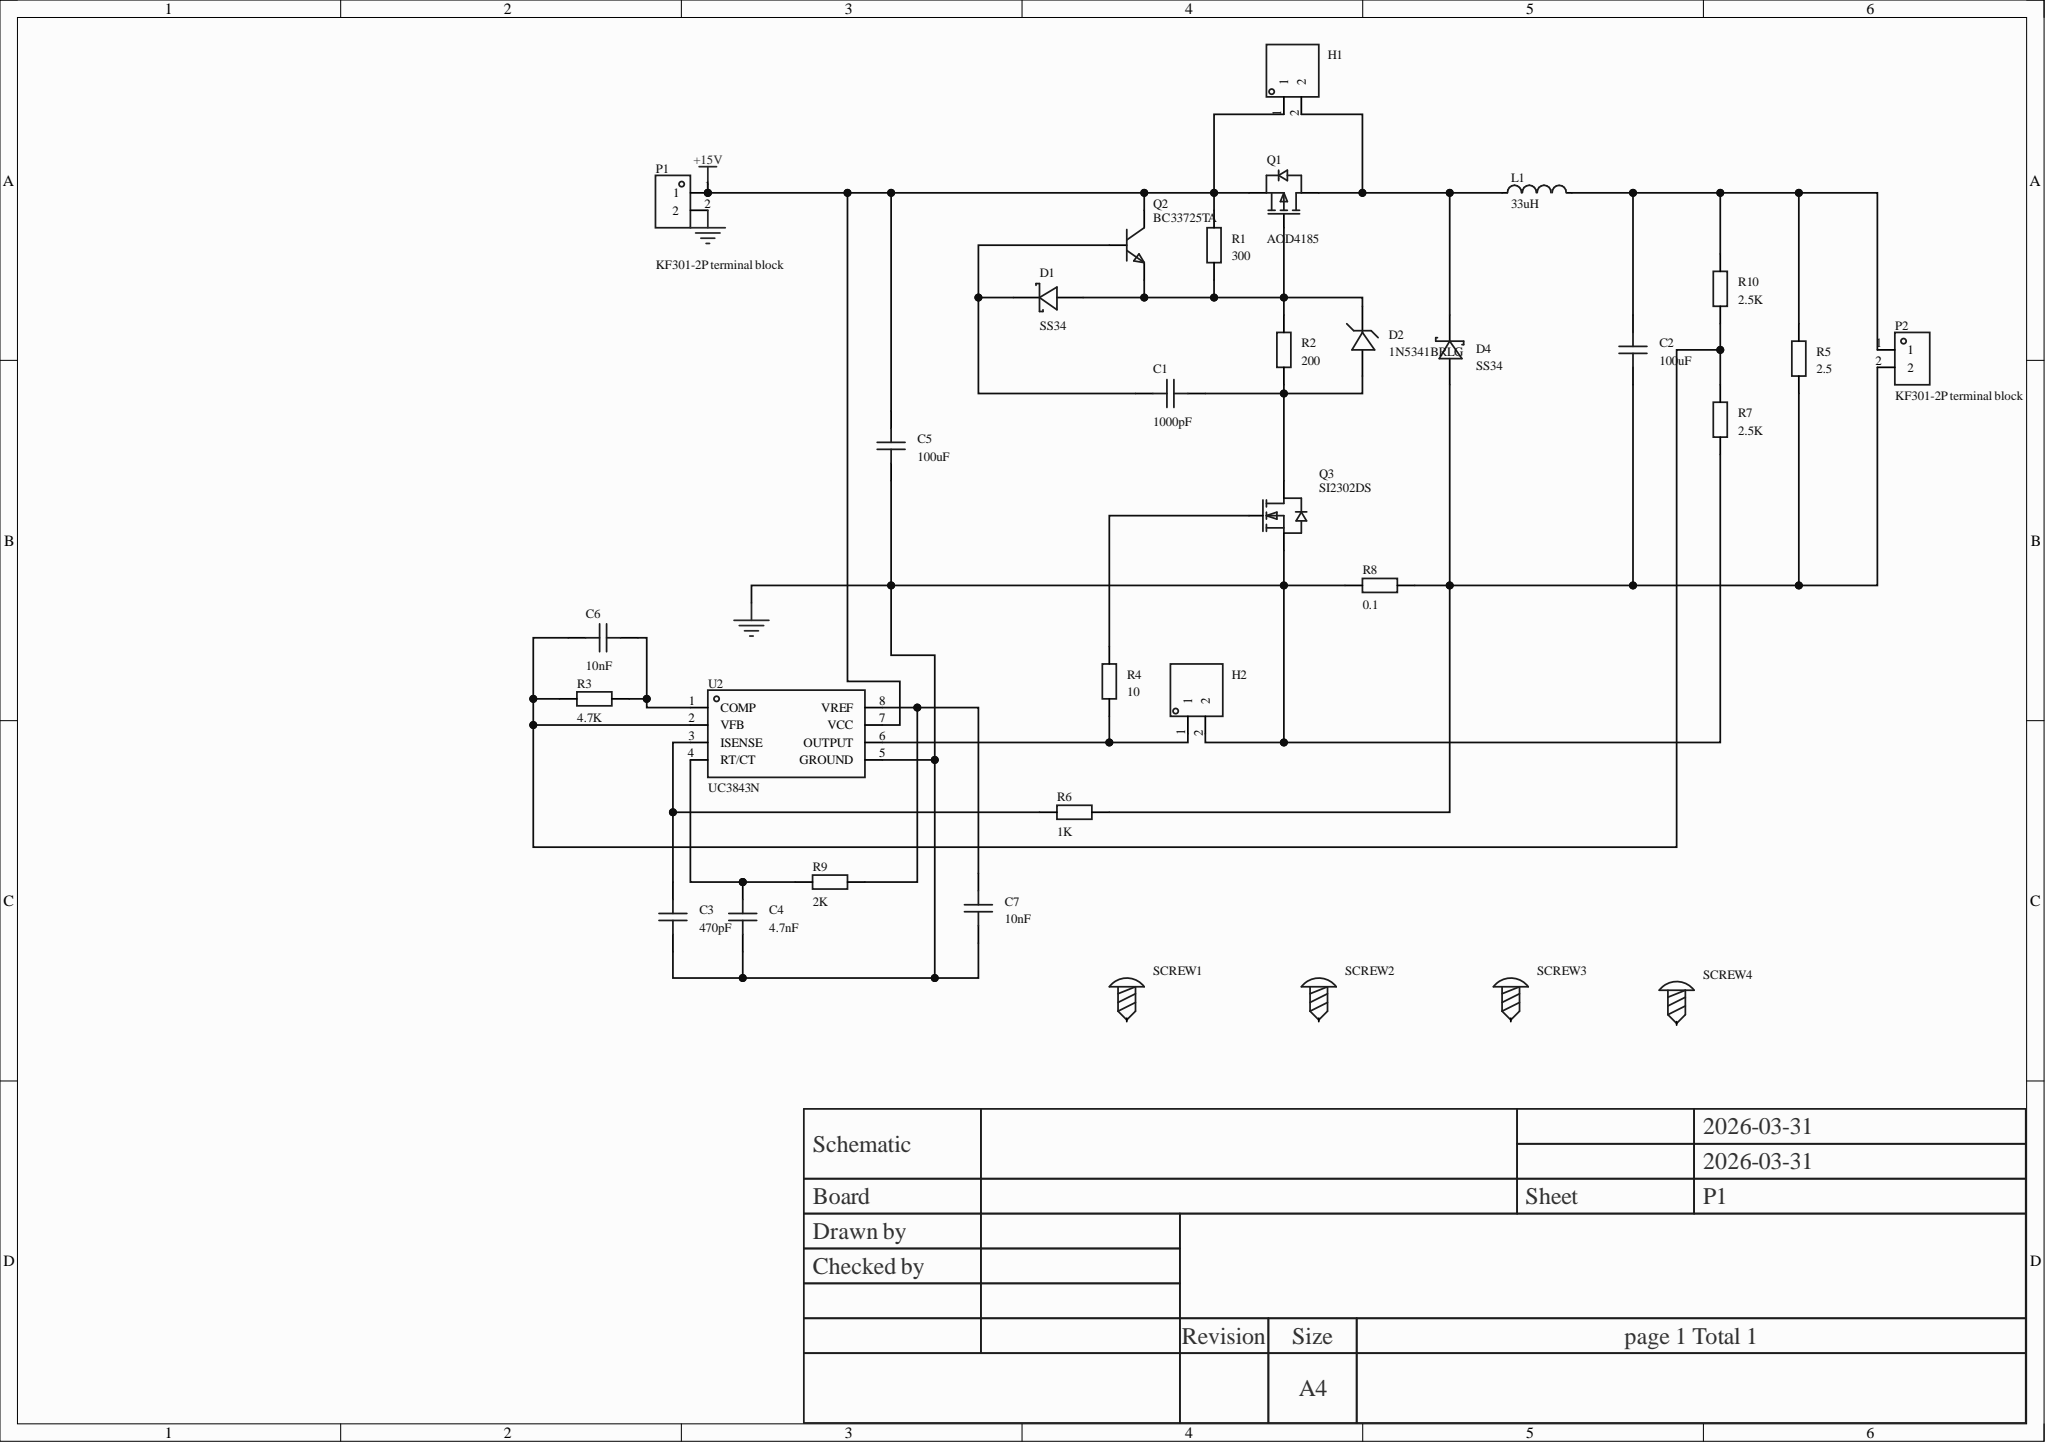Circuit board | Altium Designer | 33 parts | 15 nets
Bill of materials:
Comment,Description,Designator,Footprint,LibRef,Quantity
"1000pF","","C1","CAP-TH_L5.0-W2.5-P5.00-D1.0","CAP_0603","1"
"100uF","","C2, C5","CAP-TH_BD8.0-P3.50-D0.6-FD_1","CAP_0603","2"
"470pF","","C3","CAP-TH_L5.0-W2.5-P5.00-D1.0","CAP_0603","1"
"4.7nF","","C4","CAP-TH_L5.0-W2.5-P5.00-D1.0","CAP_0603","1"
"10nF","","C6","CAP-TH_L5.0-W2.5-P5.00-D1.0","CAP_0603","1"
"10nF","","C7","C0603","CAP_0603","1"
"SS34","Forward voltage (Vf): 500mV@3A; DC reverse voltage (Vr): 40V; Rectified current: 3A;","D1, D4","DO-15_BD3.1-L6.7-P10.70-D0.8-RD","SS34_C154551","2"
"1N5341BRLG","Diode configuration: standalone; Zener voltage (nominal): 6.2V; Zener voltage (range): 5.89V~6.51V; Tolerance: ±5%; Power: 5W; Reverse current (Ir): 1uA@3V; Impedance (Zzt): 1O;","D2","DO-15_BD3.1-L6.7-P10.70-D0.8-RD","1N5341BRLG","1"
"","","H1, H2","HDR-TH_2P-P2.54-V-M-1","HDR-M_2.54_1x2P","2"
"33uH","","L1","IND-TH_BD7.8-P5.00-D0.7","L_0603","1"
"KF301-2P terminal block","","P1, P2","CONN-TH_XY301V-A-5.0-2P","KF301-2P接线端子","2"
"AOD4185","Type: 1 P-channel; Drain-source voltage (Vdss): 40V; Continuous drain current (Id): 40A; On-resistance (RDS(on)@Vgs,Id): 20mO@4.5V,15A; Power (Pd): 62.5W; Threshold voltage (Vgs(th)@Id): 1.7V@250uA;","Q1","SOT-23-3_L2.9-W1.3-P1.90-LS2.4-L","AOD4185_C400894","1"
"BC33725TA","Transistor type: NPN; Collector current (Ic): 800mA; Collector-emitter breakdown voltage (Vceo): 45V; Power dissipation (Pd): 625mW; DC current gain (hFE): 100@100mA,1V;","Q2","TO-92-3_L4.9-W3.7-P2.54-L","BC33725TA","1"
"SI2302DS","Quantity: 1 N-channel; Drain-source voltage (Vdss): 20V; Continuous drain current (Id): 2.8A; On-resistance (RDS(on)): 120mO@2.5V; 83mO@4.5V; Power dissipation (Pd): 900mW; Threshold voltage (Vgs(th)): 1.5V;","Q3","SOT-23-3_L2.9-W1.3-P1.90-LS2.4-L","SI2302DS","1"
"300","","R1","Res_1/4W","Res_0603","1"
"200","","R2","Res_1/4W","Res_0603","1"
"4.7K","","R3","Res_1/4W","Res_0603","1"
"10","","R4","Res_1/4W","Res_0603","1"
"2.5","","R5","Res_1/4W","Res_0603","1"
"1K","","R6","Res_1/4W","Res_0603","1"
"2.5K","","R7, R10","Res_1/4W","Res_0603","2"
"0.1","","R8","Res_1/4W","Res_0603","1"
"2K","","R9","Res_1/4W","Res_0603","1"
"","","SCREW1, SCREW2, SCREW3, SCREW4","M3螺丝","M3螺丝","4"
"UC3843N","Operating voltage: 12V~28V;","U2","SOP-8_L5.1-W3.9-P1.27-LS6.0-BL","UC3843N","1"
Netlist (Protel format):
[
C1
CAP-TH_L5.0-W2.5-P5.00-D1.0
1000pF



]
[
C2
CAP-TH_BD8.0-P3.50-D0.6-FD_1
100uF



]
[
C3
CAP-TH_L5.0-W2.5-P5.00-D1.0
470pF



]
[
C4
CAP-TH_L5.0-W2.5-P5.00-D1.0
4.7nF



]
[
C5
CAP-TH_BD8.0-P3.50-D0.6-FD_1
100uF



]
[
C6
CAP-TH_L5.0-W2.5-P5.00-D1.0
10nF



]
[
C7
C0603
10nF



]
[
D1
DO-15_BD3.1-L6.7-P10.70-D0.8-RD
SS34



]
[
D2
DO-15_BD3.1-L6.7-P10.70-D0.8-RD
1N5341BRLG



]
[
D4
DO-15_BD3.1-L6.7-P10.70-D0.8-RD
SS34



]
[
H1
HDR-TH_2P-P2.54-V-M-1




]
[
H2
HDR-TH_2P-P2.54-V-M-1




]
[
L1
IND-TH_BD7.8-P5.00-D0.7
33uH



]
[
P1
CONN-TH_XY301V-A-5.0-2P
KF301-2P terminal block



]
[
P2
CONN-TH_XY301V-A-5.0-2P
KF301-2P terminal block



]
[
Q1
SOT-23-3_L2.9-W1.3-P1.90-LS2.4-L
AOD4185



]
[
Q2
TO-92-3_L4.9-W3.7-P2.54-L
BC33725TA



]
[
Q3
SOT-23-3_L2.9-W1.3-P1.90-LS2.4-L
SI2302DS



]
[
R1
Res_1/4W
300



]
[
R2
Res_1/4W
200



]
[
R3
Res_1/4W
4.7K



]
[
R4
Res_1/4W
10



]
[
R5
Res_1/4W
2.5



]
[
R6
Res_1/4W
1K



]
[
R7
Res_1/4W
2.5K



]
[
R8
Res_1/4W
0.1



]
[
R9
Res_1/4W
2K



]
[
R10
Res_1/4W
2.5K



]
[
SCREW1
M3螺丝




]
[
SCREW2
M3螺丝




]
[
SCREW3
M3螺丝




]
[
SCREW4
M3螺丝




]
[
U2
SOP-8_L5.1-W3.9-P1.27-LS6.0-BL
UC3843N



]
(
NetQ3_1
Q3-1
R4-1
)
(
NetH2_1
H2-1
R4-2
U2-6
)
(
NetD4_1
D4-1
H1-2
L1-1
Q1-2
)
(
NetD1_2
D1-2
D2-1
Q1-1
Q2-3
R1-2
R2-1
)
(
NetC7_2
C7-2
R9-2
U2-8
)
(
NetC6_2
C6-2
R3-2
U2-1
)
(
NetC6_1
C6-1
R3-1
R7-2
R10-1
U2-2
)
(
NetC4_2
C4-2
R9-1
U2-4
)
(
NetC3_2
C3-2
R6-1
U2-3
)
(
NetC2_2
C2-2
L1-2
P2-1
R5-2
R10-2
)
(
NetC2_1
C2-1
D4-2
P2-2
R5-1
R6-2
R8-2
)
(
NetC1_2
C1-2
D2-2
Q3-3
R2-2
)
(
NetC1_1
C1-1
D1-1
Q2-2
)
(
GND
C3-1
C4-1
C5-1
C7-1
H2-2
P1-2
Q3-2
R7-1
R8-1
U2-5
)
(
+15V
C5-2
H1-1
P1-1
Q1-3
Q2-1
R1-1
U2-7
)